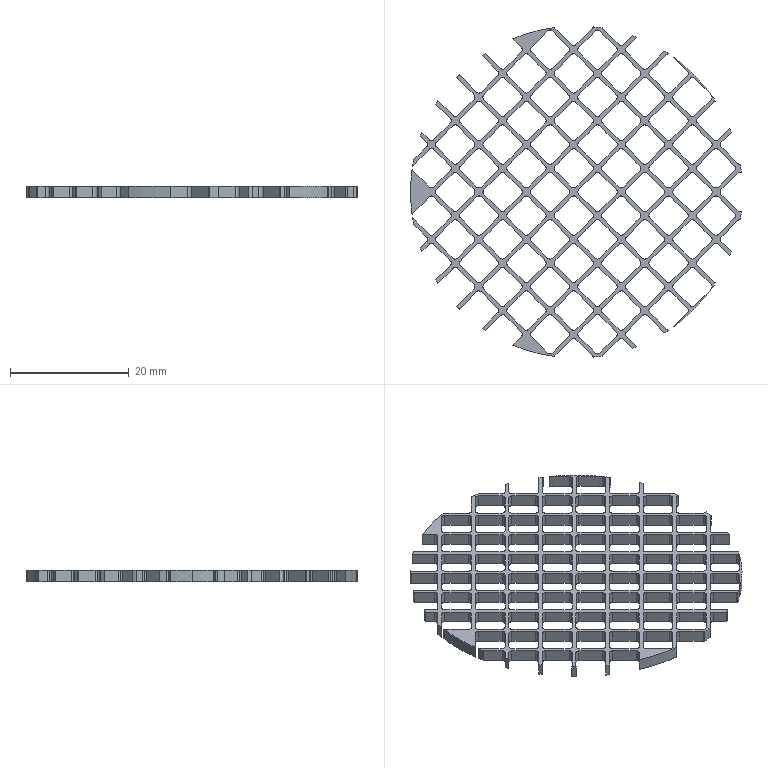Part | SolidWorks | features BaseBody 1 | 1 solid | 721 faces | box 55.811 x 55.711 x 2 mm | volume 1129 mm3 | cylinder 409 | plane 312 | commonest cylinder face diameters 1 x383 56 x26